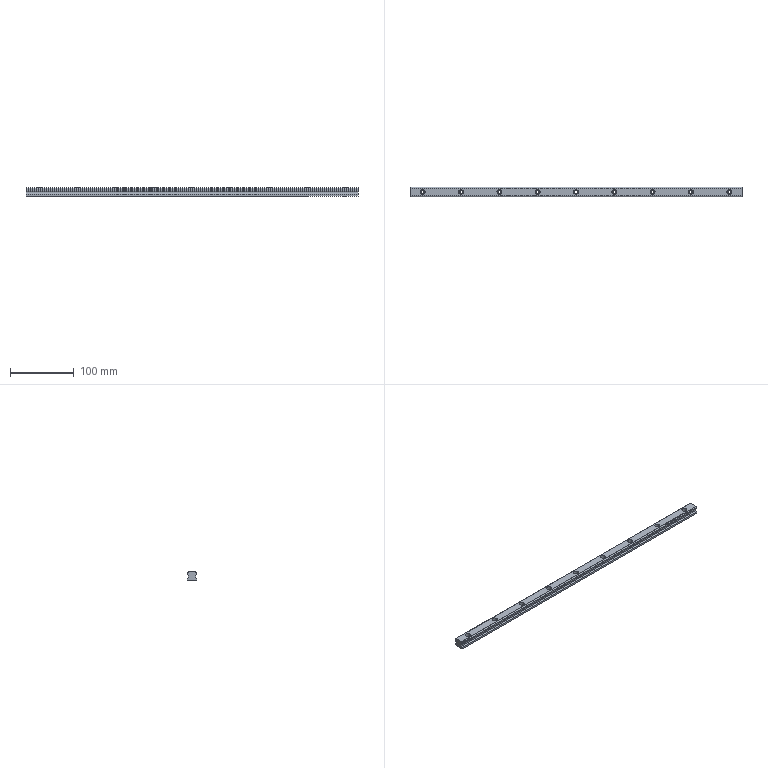Part | SolidWorks | features BaseBody 1 | 1 solid | 69 faces | box 520 x 15 x 13 mm | volume 87614 mm3 | cylinder 48 | plane 21 | commonest cylinder face diameters 4.5 x18 7.5 x18 0.28 x8 5.556 x4